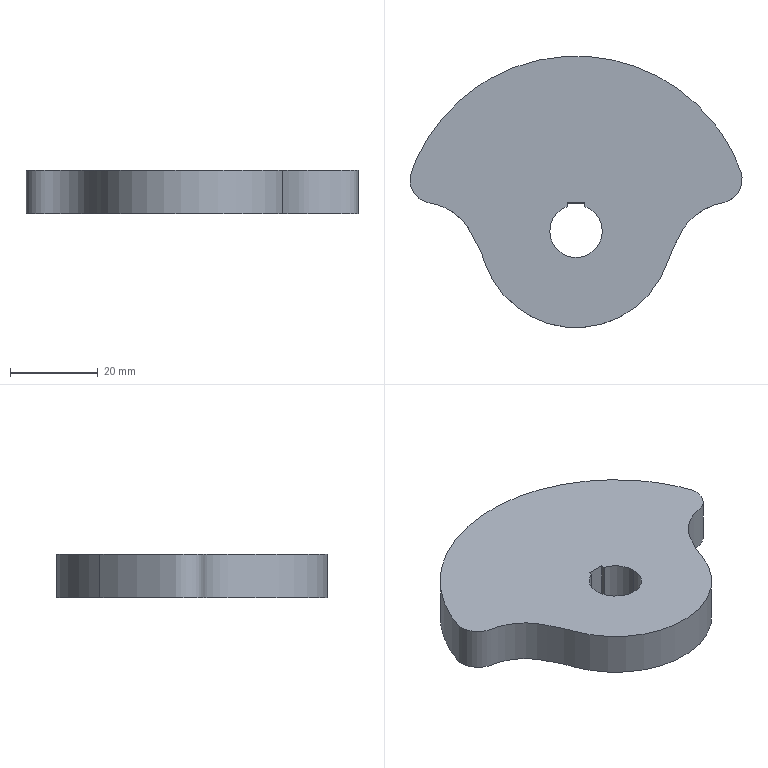Part | SolidWorks | features Extrusion 1, ICE 1 | 1 solid | 10 faces | box 75.848 x 62.021 x 10 mm | volume 30038 mm3 | plane 5 | cylinder 3 | spline 2 | commonest cylinder face diameters 12 x3
STEP:
#1=CARTESIAN_POINT('',(-6.,0.,0.));
#2=VERTEX_POINT('',#1);
#3=CARTESIAN_POINT('',(6.,0.,0.));
#4=VERTEX_POINT('',#3);
#5=CARTESIAN_POINT('',(0.,0.,0.));
#6=DIRECTION('',(0.,0.,1.));
#7=DIRECTION('',(-1.,0.,0.));
#8=AXIS2_PLACEMENT_3D('',#5,#6,#7);
#9=CIRCLE('',#8,6.);
#10=EDGE_CURVE('',#2,#4,#9,.T.);
#11=ORIENTED_EDGE('',*,*,#10,.F.);
#12=CARTESIAN_POINT('',(-6.,0.,10.));
#13=VERTEX_POINT('',#12);
#14=CARTESIAN_POINT('',(-6.,0.,-114.554));
#15=DIRECTION('',(0.,0.,1.));
#16=VECTOR('',#15,1000.);
#17=LINE('',#14,#16);
#18=EDGE_CURVE('',#2,#13,#17,.T.);
#19=ORIENTED_EDGE('',*,*,#18,.T.);
#20=CARTESIAN_POINT('',(6.,0.,10.));
#21=VERTEX_POINT('',#20);
#22=CARTESIAN_POINT('',(0.,0.,10.));
#23=DIRECTION('',(0.,0.,1.));
#24=DIRECTION('',(1.,0.,0.));
#25=AXIS2_PLACEMENT_3D('',#22,#23,#24);
#26=CIRCLE('',#25,6.);
#27=EDGE_CURVE('',#13,#21,#26,.T.);
#28=ORIENTED_EDGE('',*,*,#27,.T.);
#29=CARTESIAN_POINT('',(6.,0.,-114.554));
#30=DIRECTION('',(0.,0.,1.));
#31=VECTOR('',#30,1000.);
#32=LINE('',#29,#31);
#33=EDGE_CURVE('',#4,#21,#32,.T.);
#34=ORIENTED_EDGE('',*,*,#33,.F.);
#35=EDGE_LOOP('',(#11,#19,#28,#34));
#36=FACE_OUTER_BOUND('',#35,.T.);
#37=CARTESIAN_POINT('',(0.,0.,-114.554));
#38=DIRECTION('',(0.,0.,1.));
#39=DIRECTION('',(1.,0.,0.));
#40=AXIS2_PLACEMENT_3D('',#37,#38,#39);
#41=CYLINDRICAL_SURFACE('',#40,6.);
#42=ADVANCED_FACE('',(#36),#41,.F.);
#43=CARTESIAN_POINT('',(2.,5.657,0.));
#44=VERTEX_POINT('',#43);
#45=CARTESIAN_POINT('',(0.,0.,0.));
#46=DIRECTION('',(0.,0.,1.));
#47=DIRECTION('',(-1.,0.,0.));
#48=AXIS2_PLACEMENT_3D('',#45,#46,#47);
#49=CIRCLE('',#48,6.);
#50=EDGE_CURVE('',#4,#44,#49,.T.);
#51=ORIENTED_EDGE('',*,*,#50,.F.);
#52=ORIENTED_EDGE('',*,*,#33,.T.);
#53=CARTESIAN_POINT('',(2.,5.657,10.));
#54=VERTEX_POINT('',#53);
#55=CARTESIAN_POINT('',(0.,0.,10.));
#56=DIRECTION('',(0.,0.,1.));
#57=DIRECTION('',(1.,0.,0.));
#58=AXIS2_PLACEMENT_3D('',#55,#56,#57);
#59=CIRCLE('',#58,6.);
#60=EDGE_CURVE('',#21,#54,#59,.T.);
#61=ORIENTED_EDGE('',*,*,#60,.T.);
#62=CARTESIAN_POINT('',(2.,5.657,-114.554));
#63=DIRECTION('',(0.,0.,1.));
#64=VECTOR('',#63,1000.);
#65=LINE('',#62,#64);
#66=EDGE_CURVE('',#44,#54,#65,.T.);
#67=ORIENTED_EDGE('',*,*,#66,.F.);
#68=EDGE_LOOP('',(#51,#52,#61,#67));
#69=FACE_OUTER_BOUND('',#68,.T.);
#70=CARTESIAN_POINT('',(0.,0.,-114.554));
#71=DIRECTION('',(0.,0.,1.));
#72=DIRECTION('',(1.,0.,0.));
#73=AXIS2_PLACEMENT_3D('',#70,#71,#72);
#74=CYLINDRICAL_SURFACE('',#73,6.);
#75=ADVANCED_FACE('',(#69),#74,.F.);
#76=CARTESIAN_POINT('',(20.673,-7.557,0.));
#77=VERTEX_POINT('',#76);
#78=CARTESIAN_POINT('',(-26.47,30.003,0.));
#79=VERTEX_POINT('',#78);
#80=CARTESIAN_POINT('',(20.673,-7.557,0.));
#81=CARTESIAN_POINT('',(20.99,-6.69,0.));
#82=CARTESIAN_POINT('',(21.515,-4.914,0.));
#83=CARTESIAN_POINT('',(22.953,-2.513,0.));
#84=CARTESIAN_POINT('',(23.687,-0.8054,0.));
#85=CARTESIAN_POINT('',(24.139,-0.000000177,0.));
#86=CARTESIAN_POINT('',(25.941,3.206,0.));
#87=CARTESIAN_POINT('',(28.877,5.423,0.));
#88=CARTESIAN_POINT('',(32.454,6.278,0.));
#89=CARTESIAN_POINT('',(32.637,6.321,0.));
#90=CARTESIAN_POINT('',(33.005,6.401,0.));
#91=CARTESIAN_POINT('',(33.563,6.488,0.));
#92=CARTESIAN_POINT('',(33.928,6.581,0.));
#93=CARTESIAN_POINT('',(34.108,6.637,0.));
#94=CARTESIAN_POINT('',(36.787,7.475,0.));
#95=CARTESIAN_POINT('',(38.278,9.854,0.));
#96=CARTESIAN_POINT('',(37.865,12.63,0.));
#97=CARTESIAN_POINT('',(37.847,12.747,0.));
#98=CARTESIAN_POINT('',(37.805,12.98,0.));
#99=CARTESIAN_POINT('',(37.726,13.329,0.));
#100=CARTESIAN_POINT('',(37.646,13.552,0.));
#101=CARTESIAN_POINT('',(37.606,13.663,0.));
#102=CARTESIAN_POINT('',(37.565,13.775,0.));
#103=CARTESIAN_POINT('',(37.482,13.999,0.));
#104=CARTESIAN_POINT('',(37.355,14.334,0.));
#105=CARTESIAN_POINT('',(37.269,14.556,0.));
#106=CARTESIAN_POINT('',(37.225,14.667,0.));
#107=CARTESIAN_POINT('',(26.691,41.402,0.));
#108=CARTESIAN_POINT('',(-2.294,51.333,0.));
#109=CARTESIAN_POINT('',(-26.47,30.003,0.));
#110=(BOUNDED_CURVE()B_SPLINE_CURVE(3,(#80,#81,#82,#83,#84,#85,#86,#87,#88,#89,#90,#91,#92,#93,#94,#95,#96,#97,#98,#99,#100,#101,#102,#103,#104,#105,#106,#107,#108,#109),.UNSPECIFIED.,.F.,.F.)B_SPLINE_CURVE_WITH_KNOTS((4,1,1,3,3,1,1,3,3,1,1,3,1,1,3,4),(0.,0.01583,0.03166,0.04749,0.107,0.1102,0.1134,0.1167,0.1571,0.1591,0.1611,0.1632,0.1652,0.1672,0.1693,0.5),.UNSPECIFIED.)CURVE()GEOMETRIC_REPRESENTATION_ITEM()RATIONAL_B_SPLINE_CURVE((1.,1.,1.,1.,1.,1.,0.9442,0.9442,1.,1.,1.,1.,1.,1.,0.8399,0.8399,1.,1.,1.,1.,1.,1.,1.,1.,1.,1.,1.,0.6716,0.5986,0.7809))REPRESENTATION_ITEM(''));
#111=EDGE_CURVE('',#77,#79,#110,.T.);
#112=ORIENTED_EDGE('',*,*,#111,.T.);
#113=CARTESIAN_POINT('',(-26.47,30.003,10.));
#114=VERTEX_POINT('',#113);
#115=CARTESIAN_POINT('',(-26.47,30.003,-114.554));
#116=DIRECTION('',(0.,0.,1.));
#117=VECTOR('',#116,1000.);
#118=LINE('',#115,#117);
#119=EDGE_CURVE('',#79,#114,#118,.T.);
#120=ORIENTED_EDGE('',*,*,#119,.T.);
#121=CARTESIAN_POINT('',(20.673,-7.557,10.));
#122=VERTEX_POINT('',#121);
#123=CARTESIAN_POINT('',(20.673,-7.557,10.));
#124=CARTESIAN_POINT('',(20.99,-6.69,10.));
#125=CARTESIAN_POINT('',(21.515,-4.914,10.));
#126=CARTESIAN_POINT('',(22.953,-2.513,10.));
#127=CARTESIAN_POINT('',(23.687,-0.8054,10.));
#128=CARTESIAN_POINT('',(24.139,-0.000000177,10.));
#129=CARTESIAN_POINT('',(25.941,3.206,10.));
#130=CARTESIAN_POINT('',(28.877,5.423,10.));
#131=CARTESIAN_POINT('',(32.454,6.278,10.));
#132=CARTESIAN_POINT('',(32.637,6.321,10.));
#133=CARTESIAN_POINT('',(33.005,6.401,10.));
#134=CARTESIAN_POINT('',(33.563,6.488,10.));
#135=CARTESIAN_POINT('',(33.928,6.581,10.));
#136=CARTESIAN_POINT('',(34.108,6.637,10.));
#137=CARTESIAN_POINT('',(36.787,7.475,10.));
#138=CARTESIAN_POINT('',(38.278,9.854,10.));
#139=CARTESIAN_POINT('',(37.865,12.63,10.));
#140=CARTESIAN_POINT('',(37.847,12.747,10.));
#141=CARTESIAN_POINT('',(37.805,12.98,10.));
#142=CARTESIAN_POINT('',(37.726,13.329,10.));
#143=CARTESIAN_POINT('',(37.646,13.552,10.));
#144=CARTESIAN_POINT('',(37.606,13.663,10.));
#145=CARTESIAN_POINT('',(37.565,13.775,10.));
#146=CARTESIAN_POINT('',(37.482,13.999,10.));
#147=CARTESIAN_POINT('',(37.355,14.334,10.));
#148=CARTESIAN_POINT('',(37.269,14.556,10.));
#149=CARTESIAN_POINT('',(37.225,14.667,10.));
#150=CARTESIAN_POINT('',(26.691,41.402,10.));
#151=CARTESIAN_POINT('',(-2.294,51.333,10.));
#152=CARTESIAN_POINT('',(-26.47,30.003,10.));
#153=(BOUNDED_CURVE()B_SPLINE_CURVE(3,(#123,#124,#125,#126,#127,#128,#129,#130,#131,#132,#133,#134,#135,#136,#137,#138,#139,#140,#141,#142,#143,#144,#145,#146,#147,#148,#149,#150,#151,#152),.UNSPECIFIED.,.F.,.F.)B_SPLINE_CURVE_WITH_KNOTS((4,1,1,3,3,1,1,3,3,1,1,3,1,1,3,4),(0.,0.01583,0.03166,0.04749,0.107,0.1102,0.1134,0.1167,0.1571,0.1591,0.1611,0.1632,0.1652,0.1672,0.1693,0.5),.UNSPECIFIED.)CURVE()GEOMETRIC_REPRESENTATION_ITEM()RATIONAL_B_SPLINE_CURVE((1.,1.,1.,1.,1.,1.,0.9442,0.9442,1.,1.,1.,1.,1.,1.,0.8399,0.8399,1.,1.,1.,1.,1.,1.,1.,1.,1.,1.,1.,0.6716,0.5986,0.7809))REPRESENTATION_ITEM(''));
#154=EDGE_CURVE('',#122,#114,#153,.T.);
#155=ORIENTED_EDGE('',*,*,#154,.F.);
#156=CARTESIAN_POINT('',(20.673,-7.557,-114.554));
#157=DIRECTION('',(0.,0.,1.));
#158=VECTOR('',#157,1000.);
#159=LINE('',#156,#158);
#160=EDGE_CURVE('',#77,#122,#159,.T.);
#161=ORIENTED_EDGE('',*,*,#160,.F.);
#162=EDGE_LOOP('',(#112,#120,#155,#161));
#163=FACE_OUTER_BOUND('',#162,.T.);
#164=CARTESIAN_POINT('',(20.673,-7.557,0.));
#165=CARTESIAN_POINT('',(20.673,-7.557,10.));
#166=CARTESIAN_POINT('',(20.99,-6.69,0.));
#167=CARTESIAN_POINT('',(20.99,-6.69,10.));
#168=CARTESIAN_POINT('',(21.515,-4.914,0.));
#169=CARTESIAN_POINT('',(21.515,-4.914,10.));
#170=CARTESIAN_POINT('',(22.953,-2.513,0.));
#171=CARTESIAN_POINT('',(22.953,-2.513,10.));
#172=CARTESIAN_POINT('',(23.687,-0.8054,0.));
#173=CARTESIAN_POINT('',(23.687,-0.8054,10.));
#174=CARTESIAN_POINT('',(24.139,-0.000000177,0.));
#175=CARTESIAN_POINT('',(24.139,-0.000000177,10.));
#176=CARTESIAN_POINT('',(25.941,3.206,0.));
#177=CARTESIAN_POINT('',(25.941,3.206,10.));
#178=CARTESIAN_POINT('',(28.877,5.423,0.));
#179=CARTESIAN_POINT('',(28.877,5.423,10.));
#180=CARTESIAN_POINT('',(32.454,6.278,0.));
#181=CARTESIAN_POINT('',(32.454,6.278,10.));
#182=CARTESIAN_POINT('',(32.637,6.321,0.));
#183=CARTESIAN_POINT('',(32.637,6.321,10.));
#184=CARTESIAN_POINT('',(33.005,6.401,0.));
#185=CARTESIAN_POINT('',(33.005,6.401,10.));
#186=CARTESIAN_POINT('',(33.563,6.488,0.));
#187=CARTESIAN_POINT('',(33.563,6.488,10.));
#188=CARTESIAN_POINT('',(33.928,6.581,0.));
#189=CARTESIAN_POINT('',(33.928,6.581,10.));
#190=CARTESIAN_POINT('',(34.108,6.637,0.));
#191=CARTESIAN_POINT('',(34.108,6.637,10.));
#192=CARTESIAN_POINT('',(36.787,7.475,0.));
#193=CARTESIAN_POINT('',(36.787,7.475,10.));
#194=CARTESIAN_POINT('',(38.278,9.854,0.));
#195=CARTESIAN_POINT('',(38.278,9.854,10.));
#196=CARTESIAN_POINT('',(37.865,12.63,0.));
#197=CARTESIAN_POINT('',(37.865,12.63,10.));
#198=CARTESIAN_POINT('',(37.847,12.747,0.));
#199=CARTESIAN_POINT('',(37.847,12.747,10.));
#200=CARTESIAN_POINT('',(37.805,12.98,0.));
#201=CARTESIAN_POINT('',(37.805,12.98,10.));
#202=CARTESIAN_POINT('',(37.726,13.329,0.));
#203=CARTESIAN_POINT('',(37.726,13.329,10.));
#204=CARTESIAN_POINT('',(37.646,13.552,0.));
#205=CARTESIAN_POINT('',(37.646,13.552,10.));
#206=CARTESIAN_POINT('',(37.606,13.663,0.));
#207=CARTESIAN_POINT('',(37.606,13.663,10.));
#208=CARTESIAN_POINT('',(37.565,13.775,0.));
#209=CARTESIAN_POINT('',(37.565,13.775,10.));
#210=CARTESIAN_POINT('',(37.482,13.999,0.));
#211=CARTESIAN_POINT('',(37.482,13.999,10.));
#212=CARTESIAN_POINT('',(37.355,14.334,0.));
#213=CARTESIAN_POINT('',(37.355,14.334,10.));
#214=CARTESIAN_POINT('',(37.269,14.556,0.));
#215=CARTESIAN_POINT('',(37.269,14.556,10.));
#216=CARTESIAN_POINT('',(37.225,14.667,0.));
#217=CARTESIAN_POINT('',(37.225,14.667,10.));
#218=CARTESIAN_POINT('',(26.691,41.402,0.));
#219=CARTESIAN_POINT('',(26.691,41.402,10.));
#220=CARTESIAN_POINT('',(-2.294,51.333,0.));
#221=CARTESIAN_POINT('',(-2.294,51.333,10.));
#222=CARTESIAN_POINT('',(-26.47,30.003,0.));
#223=CARTESIAN_POINT('',(-26.47,30.003,10.));
#224=(BOUNDED_SURFACE()B_SPLINE_SURFACE(3,1,((#164,#165),(#166,#167),(#168,#169),(#170,#171),(#172,#173),(#174,#175),(#176,#177),(#178,#179),(#180,#181),(#182,#183),(#184,#185),(#186,#187),(#188,#189),(#190,#191),(#192,#193),(#194,#195),(#196,#197),(#198,#199),(#200,#201),(#202,#203),(#204,#205),(#206,#207),(#208,#209),(#210,#211),(#212,#213),(#214,#215),(#216,#217),(#218,#219),(#220,#221),(#222,#223)),.UNSPECIFIED.,.F.,.F.,.F.)B_SPLINE_SURFACE_WITH_KNOTS((4,1,1,3,3,1,1,3,3,1,1,3,1,1,3,4),(2,2),(0.,0.01583,0.03166,0.04749,0.107,0.1102,0.1134,0.1167,0.1571,0.1591,0.1611,0.1632,0.1652,0.1672,0.1693,0.5),(0.,1.),.UNSPECIFIED.)GEOMETRIC_REPRESENTATION_ITEM()RATIONAL_B_SPLINE_SURFACE(((1.,1.),(1.,1.),(1.,1.),(1.,1.),(1.,1.),(1.,1.),(0.9442,0.9442),(0.9442,0.9442),(1.,1.),(1.,1.),(1.,1.),(1.,1.),(1.,1.),(1.,1.),(0.8399,0.8399),(0.8399,0.8399),(1.,1.),(1.,1.),(1.,1.),(1.,1.),(1.,1.),(1.,1.),(1.,1.),(1.,1.),(1.,1.),(1.,1.),(1.,1.),(0.6716,0.6716),(0.5986,0.5986),(0.7809,0.7809)))REPRESENTATION_ITEM('')SURFACE());
#225=ADVANCED_FACE('',(#163),#224,.T.);
#226=ORIENTED_EDGE('',*,*,#119,.F.);
#227=CARTESIAN_POINT('',(-26.47,30.003,0.));
#228=CARTESIAN_POINT('',(-31.437,25.621,0.));
#229=CARTESIAN_POINT('',(-34.994,20.332,0.));
#230=CARTESIAN_POINT('',(-37.226,14.666,0.));
#231=CARTESIAN_POINT('',(-37.27,14.555,0.));
#232=CARTESIAN_POINT('',(-37.356,14.333,0.));
#233=CARTESIAN_POINT('',(-37.483,13.998,0.));
#234=CARTESIAN_POINT('',(-37.565,13.775,0.));
#235=CARTESIAN_POINT('',(-37.606,13.663,0.));
#236=CARTESIAN_POINT('',(-37.646,13.552,0.));
#237=CARTESIAN_POINT('',(-37.726,13.329,0.));
#238=CARTESIAN_POINT('',(-37.805,12.981,0.));
#239=CARTESIAN_POINT('',(-37.847,12.748,0.));
#240=CARTESIAN_POINT('',(-37.864,12.631,0.));
#241=CARTESIAN_POINT('',(-38.279,9.854,0.));
#242=CARTESIAN_POINT('',(-36.787,7.475,0.));
#243=CARTESIAN_POINT('',(-34.108,6.637,0.));
#244=CARTESIAN_POINT('',(-33.928,6.581,0.));
#245=CARTESIAN_POINT('',(-33.563,6.488,0.));
#246=CARTESIAN_POINT('',(-33.005,6.401,0.));
#247=CARTESIAN_POINT('',(-32.637,6.321,0.));
#248=CARTESIAN_POINT('',(-32.454,6.278,0.));
#249=CARTESIAN_POINT('',(-28.877,5.423,0.));
#250=CARTESIAN_POINT('',(-25.941,3.206,0.));
#251=CARTESIAN_POINT('',(-24.139,0.,0.));
#252=CARTESIAN_POINT('',(-23.687,-0.8052,0.));
#253=CARTESIAN_POINT('',(-22.953,-2.512,0.));
#254=CARTESIAN_POINT('',(-21.515,-4.913,0.));
#255=CARTESIAN_POINT('',(-20.99,-6.688,0.));
#256=CARTESIAN_POINT('',(-20.673,-7.556,0.));
#257=CARTESIAN_POINT('',(-12.258,-30.58,0.));
#258=CARTESIAN_POINT('',(12.256,-30.581,0.));
#259=CARTESIAN_POINT('',(20.673,-7.557,0.));
#260=(BOUNDED_CURVE()B_SPLINE_CURVE(3,(#227,#228,#229,#230,#231,#232,#233,#234,#235,#236,#237,#238,#239,#240,#241,#242,#243,#244,#245,#246,#247,#248,#249,#250,#251,#252,#253,#254,#255,#256,#257,#258,#259),.UNSPECIFIED.,.F.,.T.)B_SPLINE_CURVE_WITH_KNOTS((4,3,1,1,3,1,1,3,3,1,1,3,3,1,1,3,4),(0.5,0.5946,0.5966,0.5986,0.6007,0.6027,0.6047,0.6068,0.6472,0.6504,0.6536,0.6568,0.7163,0.7322,0.748,0.7638,1.),.UNSPECIFIED.)CURVE()GEOMETRIC_REPRESENTATION_ITEM()RATIONAL_B_SPLINE_CURVE((0.7809,0.8331,0.9061,1.,1.,1.,1.,1.,1.,1.,1.,1.,1.,1.,0.8398,0.8398,1.,1.,1.,1.,1.,1.,0.9442,0.9442,1.,1.,1.,1.,1.,1.,0.5622,0.5622,1.))REPRESENTATION_ITEM(''));
#261=EDGE_CURVE('',#79,#77,#260,.T.);
#262=ORIENTED_EDGE('',*,*,#261,.T.);
#263=ORIENTED_EDGE('',*,*,#160,.T.);
#264=CARTESIAN_POINT('',(-26.47,30.003,10.));
#265=CARTESIAN_POINT('',(-31.437,25.621,10.));
#266=CARTESIAN_POINT('',(-34.994,20.332,10.));
#267=CARTESIAN_POINT('',(-37.226,14.666,10.));
#268=CARTESIAN_POINT('',(-37.27,14.555,10.));
#269=CARTESIAN_POINT('',(-37.356,14.333,10.));
#270=CARTESIAN_POINT('',(-37.483,13.998,10.));
#271=CARTESIAN_POINT('',(-37.565,13.775,10.));
#272=CARTESIAN_POINT('',(-37.606,13.663,10.));
#273=CARTESIAN_POINT('',(-37.646,13.552,10.));
#274=CARTESIAN_POINT('',(-37.726,13.329,10.));
#275=CARTESIAN_POINT('',(-37.805,12.981,10.));
#276=CARTESIAN_POINT('',(-37.847,12.748,10.));
#277=CARTESIAN_POINT('',(-37.864,12.631,10.));
#278=CARTESIAN_POINT('',(-38.279,9.854,10.));
#279=CARTESIAN_POINT('',(-36.787,7.475,10.));
#280=CARTESIAN_POINT('',(-34.108,6.637,10.));
#281=CARTESIAN_POINT('',(-33.928,6.581,10.));
#282=CARTESIAN_POINT('',(-33.563,6.488,10.));
#283=CARTESIAN_POINT('',(-33.005,6.401,10.));
#284=CARTESIAN_POINT('',(-32.637,6.321,10.));
#285=CARTESIAN_POINT('',(-32.454,6.278,10.));
#286=CARTESIAN_POINT('',(-28.877,5.423,10.));
#287=CARTESIAN_POINT('',(-25.941,3.206,10.));
#288=CARTESIAN_POINT('',(-24.139,0.,10.));
#289=CARTESIAN_POINT('',(-23.687,-0.8052,10.));
#290=CARTESIAN_POINT('',(-22.953,-2.512,10.));
#291=CARTESIAN_POINT('',(-21.515,-4.913,10.));
#292=CARTESIAN_POINT('',(-20.99,-6.688,10.));
#293=CARTESIAN_POINT('',(-20.673,-7.556,10.));
#294=CARTESIAN_POINT('',(-12.258,-30.58,10.));
#295=CARTESIAN_POINT('',(12.256,-30.581,10.));
#296=CARTESIAN_POINT('',(20.673,-7.557,10.));
#297=(BOUNDED_CURVE()B_SPLINE_CURVE(3,(#264,#265,#266,#267,#268,#269,#270,#271,#272,#273,#274,#275,#276,#277,#278,#279,#280,#281,#282,#283,#284,#285,#286,#287,#288,#289,#290,#291,#292,#293,#294,#295,#296),.UNSPECIFIED.,.F.,.F.)B_SPLINE_CURVE_WITH_KNOTS((4,3,1,1,3,1,1,3,3,1,1,3,3,1,1,3,4),(0.5,0.5946,0.5966,0.5986,0.6007,0.6027,0.6047,0.6068,0.6472,0.6504,0.6536,0.6568,0.7163,0.7322,0.748,0.7638,1.),.UNSPECIFIED.)CURVE()GEOMETRIC_REPRESENTATION_ITEM()RATIONAL_B_SPLINE_CURVE((0.7809,0.8331,0.9061,1.,1.,1.,1.,1.,1.,1.,1.,1.,1.,1.,0.8398,0.8398,1.,1.,1.,1.,1.,1.,0.9442,0.9442,1.,1.,1.,1.,1.,1.,0.5622,0.5622,1.))REPRESENTATION_ITEM(''));
#298=EDGE_CURVE('',#114,#122,#297,.T.);
#299=ORIENTED_EDGE('',*,*,#298,.F.);
#300=EDGE_LOOP('',(#226,#262,#263,#299));
#301=FACE_OUTER_BOUND('',#300,.T.);
#302=CARTESIAN_POINT('',(-26.47,30.003,0.));
#303=CARTESIAN_POINT('',(-26.47,30.003,10.));
#304=CARTESIAN_POINT('',(-31.437,25.621,0.));
#305=CARTESIAN_POINT('',(-31.437,25.621,10.));
#306=CARTESIAN_POINT('',(-34.994,20.332,0.));
#307=CARTESIAN_POINT('',(-34.994,20.332,10.));
#308=CARTESIAN_POINT('',(-37.226,14.666,0.));
#309=CARTESIAN_POINT('',(-37.226,14.666,10.));
#310=CARTESIAN_POINT('',(-37.27,14.555,0.));
#311=CARTESIAN_POINT('',(-37.27,14.555,10.));
#312=CARTESIAN_POINT('',(-37.356,14.333,0.));
#313=CARTESIAN_POINT('',(-37.356,14.333,10.));
#314=CARTESIAN_POINT('',(-37.483,13.998,0.));
#315=CARTESIAN_POINT('',(-37.483,13.998,10.));
#316=CARTESIAN_POINT('',(-37.565,13.775,0.));
#317=CARTESIAN_POINT('',(-37.565,13.775,10.));
#318=CARTESIAN_POINT('',(-37.606,13.663,0.));
#319=CARTESIAN_POINT('',(-37.606,13.663,10.));
#320=CARTESIAN_POINT('',(-37.646,13.552,0.));
#321=CARTESIAN_POINT('',(-37.646,13.552,10.));
#322=CARTESIAN_POINT('',(-37.726,13.329,0.));
#323=CARTESIAN_POINT('',(-37.726,13.329,10.));
#324=CARTESIAN_POINT('',(-37.805,12.981,0.));
#325=CARTESIAN_POINT('',(-37.805,12.981,10.));
#326=CARTESIAN_POINT('',(-37.847,12.748,0.));
#327=CARTESIAN_POINT('',(-37.847,12.748,10.));
#328=CARTESIAN_POINT('',(-37.864,12.631,0.));
#329=CARTESIAN_POINT('',(-37.864,12.631,10.));
#330=CARTESIAN_POINT('',(-38.279,9.854,0.));
#331=CARTESIAN_POINT('',(-38.279,9.854,10.));
#332=CARTESIAN_POINT('',(-36.787,7.475,0.));
#333=CARTESIAN_POINT('',(-36.787,7.475,10.));
#334=CARTESIAN_POINT('',(-34.108,6.637,0.));
#335=CARTESIAN_POINT('',(-34.108,6.637,10.));
#336=CARTESIAN_POINT('',(-33.928,6.581,0.));
#337=CARTESIAN_POINT('',(-33.928,6.581,10.));
#338=CARTESIAN_POINT('',(-33.563,6.488,0.));
#339=CARTESIAN_POINT('',(-33.563,6.488,10.));
#340=CARTESIAN_POINT('',(-33.005,6.401,0.));
#341=CARTESIAN_POINT('',(-33.005,6.401,10.));
#342=CARTESIAN_POINT('',(-32.637,6.321,0.));
#343=CARTESIAN_POINT('',(-32.637,6.321,10.));
#344=CARTESIAN_POINT('',(-32.454,6.278,0.));
#345=CARTESIAN_POINT('',(-32.454,6.278,10.));
#346=CARTESIAN_POINT('',(-28.877,5.423,0.));
#347=CARTESIAN_POINT('',(-28.877,5.423,10.));
#348=CARTESIAN_POINT('',(-25.941,3.206,0.));
#349=CARTESIAN_POINT('',(-25.941,3.206,10.));
#350=CARTESIAN_POINT('',(-24.139,0.,0.));
#351=CARTESIAN_POINT('',(-24.139,0.,10.));
#352=CARTESIAN_POINT('',(-23.687,-0.8052,0.));
#353=CARTESIAN_POINT('',(-23.687,-0.8052,10.));
#354=CARTESIAN_POINT('',(-22.953,-2.512,0.));
#355=CARTESIAN_POINT('',(-22.953,-2.512,10.));
#356=CARTESIAN_POINT('',(-21.515,-4.913,0.));
#357=CARTESIAN_POINT('',(-21.515,-4.913,10.));
#358=CARTESIAN_POINT('',(-20.99,-6.688,0.));
#359=CARTESIAN_POINT('',(-20.99,-6.688,10.));
#360=CARTESIAN_POINT('',(-20.673,-7.556,0.));
#361=CARTESIAN_POINT('',(-20.673,-7.556,10.));
#362=CARTESIAN_POINT('',(-12.258,-30.58,0.));
#363=CARTESIAN_POINT('',(-12.258,-30.58,10.));
#364=CARTESIAN_POINT('',(12.256,-30.581,0.));
#365=CARTESIAN_POINT('',(12.256,-30.581,10.));
#366=CARTESIAN_POINT('',(20.673,-7.557,0.));
#367=CARTESIAN_POINT('',(20.673,-7.557,10.));
#368=(BOUNDED_SURFACE()B_SPLINE_SURFACE(3,1,((#302,#303),(#304,#305),(#306,#307),(#308,#309),(#310,#311),(#312,#313),(#314,#315),(#316,#317),(#318,#319),(#320,#321),(#322,#323),(#324,#325),(#326,#327),(#328,#329),(#330,#331),(#332,#333),(#334,#335),(#336,#337),(#338,#339),(#340,#341),(#342,#343),(#344,#345),(#346,#347),(#348,#349),(#350,#351),(#352,#353),(#354,#355),(#356,#357),(#358,#359),(#360,#361),(#362,#363),(#364,#365),(#366,#367)),.UNSPECIFIED.,.F.,.F.,.T.)B_SPLINE_SURFACE_WITH_KNOTS((4,3,1,1,3,1,1,3,3,1,1,3,3,1,1,3,4),(2,2),(0.5,0.5946,0.5966,0.5986,0.6007,0.6027,0.6047,0.6068,0.6472,0.6504,0.6536,0.6568,0.7163,0.7322,0.748,0.7638,1.),(0.,1.),.UNSPECIFIED.)GEOMETRIC_REPRESENTATION_ITEM()RATIONAL_B_SPLINE_SURFACE(((0.7809,0.7809),(0.8331,0.8331),(0.9061,0.9061),(1.,1.),(1.,1.),(1.,1.),(1.,1.),(1.,1.),(1.,1.),(1.,1.),(1.,1.),(1.,1.),(1.,1.),(1.,1.),(0.8398,0.8398),(0.8398,0.8398),(1.,1.),(1.,1.),(1.,1.),(1.,1.),(1.,1.),(1.,1.),(0.9442,0.9442),(0.9442,0.9442),(1.,1.),(1.,1.),(1.,1.),(1.,1.),(1.,1.),(1.,1.),(0.5622,0.5622),(0.5622,0.5622),(1.,1.)))REPRESENTATION_ITEM('')SURFACE());
#369=ADVANCED_FACE('',(#301),#368,.T.);
#370=CARTESIAN_POINT('',(2.,6.472,0.));
#371=VERTEX_POINT('',#370);
#372=CARTESIAN_POINT('',(-2.,6.472,0.));
#373=VERTEX_POINT('',#372);
#374=CARTESIAN_POINT('',(2.,6.472,0.));
#375=DIRECTION('',(-1.,0.,0.));
#376=VECTOR('',#375,1000.);
#377=LINE('',#374,#376);
#378=EDGE_CURVE('',#371,#373,#377,.T.);
#379=ORIENTED_EDGE('',*,*,#378,.F.);
#380=CARTESIAN_POINT('',(2.,6.472,10.));
#381=VERTEX_POINT('',#380);
#382=CARTESIAN_POINT('',(2.,6.472,-114.554));
#383=DIRECTION('',(0.,0.,1.));
#384=VECTOR('',#383,1000.);
#385=LINE('',#382,#384);
#386=EDGE_CURVE('',#371,#381,#385,.T.);
#387=ORIENTED_EDGE('',*,*,#386,.T.);
#388=CARTESIAN_POINT('',(-2.,6.472,10.));
#389=VERTEX_POINT('',#388);
#390=CARTESIAN_POINT('',(2.,6.472,10.));
#391=DIRECTION('',(-1.,0.,0.));
#392=VECTOR('',#391,1000.);
#393=LINE('',#390,#392);
#394=EDGE_CURVE('',#381,#389,#393,.T.);
#395=ORIENTED_EDGE('',*,*,#394,.T.);
#396=CARTESIAN_POINT('',(-2.,6.472,-114.554));
#397=DIRECTION('',(0.,0.,1.));
#398=VECTOR('',#397,1000.);
#399=LINE('',#396,#398);
#400=EDGE_CURVE('',#373,#389,#399,.T.);
#401=ORIENTED_EDGE('',*,*,#400,.F.);
#402=EDGE_LOOP('',(#379,#387,#395,#401));
#403=FACE_OUTER_BOUND('',#402,.T.);
#404=CARTESIAN_POINT('',(2.,6.472,-114.554));
#405=DIRECTION('',(0.,1.,0.));
#406=DIRECTION('',(-1.,0.,0.));
#407=AXIS2_PLACEMENT_3D('',#404,#405,#406);
#408=PLANE('',#407);
#409=ADVANCED_FACE('',(#403),#408,.F.);
#410=CARTESIAN_POINT('',(2.,5.657,0.));
#411=DIRECTION('',(0.,1.,0.));
#412=VECTOR('',#411,1000.);
#413=LINE('',#410,#412);
#414=EDGE_CURVE('',#44,#371,#413,.T.);
#415=ORIENTED_EDGE('',*,*,#414,.F.);
#416=ORIENTED_EDGE('',*,*,#66,.T.);
#417=CARTESIAN_POINT('',(2.,5.657,10.));
#418=DIRECTION('',(0.,1.,0.));
#419=VECTOR('',#418,1000.);
#420=LINE('',#417,#419);
#421=EDGE_CURVE('',#54,#381,#420,.T.);
#422=ORIENTED_EDGE('',*,*,#421,.T.);
#423=ORIENTED_EDGE('',*,*,#386,.F.);
#424=EDGE_LOOP('',(#415,#416,#422,#423));
#425=FACE_OUTER_BOUND('',#424,.T.);
#426=CARTESIAN_POINT('',(2.,5.657,-114.554));
#427=DIRECTION('',(1.,0.,0.));
#428=DIRECTION('',(0.,0.,-1.));
#429=AXIS2_PLACEMENT_3D('',#426,#427,#428);
#430=PLANE('',#429);
#431=ADVANCED_FACE('',(#425),#430,.F.);
#432=ORIENTED_EDGE('',*,*,#18,.F.);
#433=CARTESIAN_POINT('',(-2.,5.657,0.));
#434=VERTEX_POINT('',#433);
#435=CARTESIAN_POINT('',(0.,0.,0.));
#436=DIRECTION('',(0.,0.,1.));
#437=DIRECTION('',(-1.,0.,0.));
#438=AXIS2_PLACEMENT_3D('',#435,#436,#437);
#439=CIRCLE('',#438,6.);
#440=EDGE_CURVE('',#434,#2,#439,.T.);
#441=ORIENTED_EDGE('',*,*,#440,.F.);
#442=CARTESIAN_POINT('',(-2.,5.657,10.));
#443=VERTEX_POINT('',#442);
#444=CARTESIAN_POINT('',(-2.,5.657,-114.554));
#445=DIRECTION('',(0.,0.,1.));
#446=VECTOR('',#445,1000.);
#447=LINE('',#444,#446);
#448=EDGE_CURVE('',#434,#443,#447,.T.);
#449=ORIENTED_EDGE('',*,*,#448,.T.);
#450=CARTESIAN_POINT('',(0.,0.,10.));
#451=DIRECTION('',(0.,0.,1.));
#452=DIRECTION('',(1.,0.,0.));
#453=AXIS2_PLACEMENT_3D('',#450,#451,#452);
#454=CIRCLE('',#453,6.);
#455=EDGE_CURVE('',#443,#13,#454,.T.);
#456=ORIENTED_EDGE('',*,*,#455,.T.);
#457=EDGE_LOOP('',(#432,#441,#449,#456));
#458=FACE_OUTER_BOUND('',#457,.T.);
#459=CARTESIAN_POINT('',(0.,0.,-114.554));
#460=DIRECTION('',(0.,0.,1.));
#461=DIRECTION('',(1.,0.,0.));
#462=AXIS2_PLACEMENT_3D('',#459,#460,#461);
#463=CYLINDRICAL_SURFACE('',#462,6.);
#464=ADVANCED_FACE('',(#458),#463,.F.);
#465=CARTESIAN_POINT('',(-2.,6.472,0.));
#466=DIRECTION('',(0.,-1.,0.));
#467=VECTOR('',#466,1000.);
#468=LINE('',#465,#467);
#469=EDGE_CURVE('',#373,#434,#468,.T.);
#470=ORIENTED_EDGE('',*,*,#469,.F.);
#471=ORIENTED_EDGE('',*,*,#400,.T.);
#472=CARTESIAN_POINT('',(-2.,6.472,10.));
#473=DIRECTION('',(0.,-1.,0.));
#474=VECTOR('',#473,1000.);
#475=LINE('',#472,#474);
#476=EDGE_CURVE('',#389,#443,#475,.T.);
#477=ORIENTED_EDGE('',*,*,#476,.T.);
#478=ORIENTED_EDGE('',*,*,#448,.F.);
#479=EDGE_LOOP('',(#470,#471,#477,#478));
#480=FACE_OUTER_BOUND('',#479,.T.);
#481=CARTESIAN_POINT('',(-2.,6.472,-114.554));
#482=DIRECTION('',(-1.,0.,0.));
#483=DIRECTION('',(0.,-1.,0.));
#484=AXIS2_PLACEMENT_3D('',#481,#482,#483);
#485=PLANE('',#484);
#486=ADVANCED_FACE('',(#480),#485,.F.);
#487=ORIENTED_EDGE('',*,*,#394,.F.);
#488=ORIENTED_EDGE('',*,*,#421,.F.);
#489=ORIENTED_EDGE('',*,*,#60,.F.);
#490=ORIENTED_EDGE('',*,*,#27,.F.);
#491=ORIENTED_EDGE('',*,*,#455,.F.);
#492=ORIENTED_EDGE('',*,*,#476,.F.);
#493=EDGE_LOOP('',(#487,#488,#489,#490,#491,#492));
#494=FACE_BOUND('',#493,.T.);
#495=ORIENTED_EDGE('',*,*,#154,.T.);
#496=ORIENTED_EDGE('',*,*,#298,.T.);
#497=EDGE_LOOP('',(#495,#496));
#498=FACE_OUTER_BOUND('',#497,.T.);
#499=CARTESIAN_POINT('',(-26.47,30.003,10.));
#500=DIRECTION('',(0.,0.,1.));
#501=DIRECTION('',(1.,0.,0.));
#502=AXIS2_PLACEMENT_3D('',#499,#500,#501);
#503=PLANE('',#502);
#504=ADVANCED_FACE('',(#494,#498),#503,.T.);
#505=ORIENTED_EDGE('',*,*,#111,.F.);
#506=ORIENTED_EDGE('',*,*,#261,.F.);
#507=EDGE_LOOP('',(#505,#506));
#508=FACE_OUTER_BOUND('',#507,.T.);
#509=ORIENTED_EDGE('',*,*,#414,.T.);
#510=ORIENTED_EDGE('',*,*,#378,.T.);
#511=ORIENTED_EDGE('',*,*,#469,.T.);
#512=ORIENTED_EDGE('',*,*,#440,.T.);
#513=ORIENTED_EDGE('',*,*,#10,.T.);
#514=ORIENTED_EDGE('',*,*,#50,.T.);
#515=EDGE_LOOP('',(#509,#510,#511,#512,#513,#514));
#516=FACE_BOUND('',#515,.T.);
#517=CARTESIAN_POINT('',(-34.303,-12.485,0.));
#518=DIRECTION('',(0.,0.,-1.));
#519=DIRECTION('',(-1.,0.,0.));
#520=AXIS2_PLACEMENT_3D('',#517,#518,#519);
#521=PLANE('',#520);
#522=ADVANCED_FACE('',(#508,#516),#521,.T.);
#523=CLOSED_SHELL('',(#42,#75,#225,#369,#409,#431,#464,#486,#504,#522));
#524=MANIFOLD_SOLID_BREP('',#523);
#525=CARTESIAN_POINT('',(0.,0.,0.));
#526=DIRECTION('',(0.,0.,1.));
#527=DIRECTION('',(1.,0.,0.));
#528=AXIS2_PLACEMENT_3D('',#525,#526,#527);
#529=(LENGTH_UNIT()NAMED_UNIT(*)SI_UNIT(.MILLI.,.METRE.));
#530=UNCERTAINTY_MEASURE_WITH_UNIT(LENGTH_MEASURE(0.00001),#529,'','');
#531=(NAMED_UNIT(*)PLANE_ANGLE_UNIT()SI_UNIT($,.RADIAN.));
#532=(NAMED_UNIT(*)SI_UNIT($,.STERADIAN.)SOLID_ANGLE_UNIT());
#533=(GEOMETRIC_REPRESENTATION_CONTEXT(3)GLOBAL_UNCERTAINTY_ASSIGNED_CONTEXT((#530))GLOBAL_UNIT_ASSIGNED_CONTEXT((#529,#531,#532))REPRESENTATION_CONTEXT('',''));
#534=ADVANCED_BREP_SHAPE_REPRESENTATION('',(#524,#528),#533);